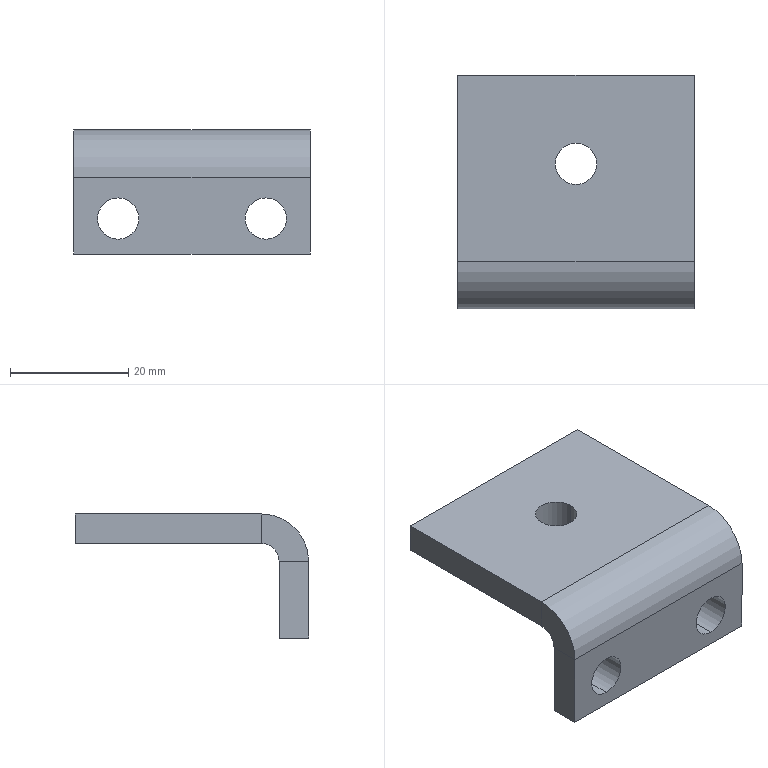Part | SolidWorks | features ICE 2, EdgeFlange 1, Fillet 1, FlatPattern 1, SMBaseFlange 1, SheetMetal 1 | 1 solid | 20 faces | box 40 x 39.5 x 21 mm | volume 10051 mm3 | plane 12 | cylinder 8 | commonest cylinder face diameters 7 x6 6 x1 16 x1
STEP:
#1=CARTESIAN_POINT('',(12.5,-5.,-8.));
#2=VERTEX_POINT('',#1);
#3=CARTESIAN_POINT('',(12.5,-5.,-1.));
#4=VERTEX_POINT('',#3);
#5=CARTESIAN_POINT('',(12.5,-5.,-4.5));
#6=DIRECTION('',(0.,1.,0.));
#7=DIRECTION('',(0.,0.,1.));
#8=AXIS2_PLACEMENT_3D('',#5,#6,#7);
#9=CIRCLE('',#8,3.5);
#10=EDGE_CURVE('',#2,#4,#9,.T.);
#11=ORIENTED_EDGE('',*,*,#10,.F.);
#12=CARTESIAN_POINT('',(12.5,0.,-8.));
#13=VERTEX_POINT('',#12);
#14=CARTESIAN_POINT('',(12.5,-5.,-8.));
#15=DIRECTION('',(0.,1.,0.));
#16=VECTOR('',#15,1000.);
#17=LINE('',#14,#16);
#18=EDGE_CURVE('',#2,#13,#17,.T.);
#19=ORIENTED_EDGE('',*,*,#18,.T.);
#20=CARTESIAN_POINT('',(12.5,0.,-1.));
#21=VERTEX_POINT('',#20);
#22=CARTESIAN_POINT('',(12.5,0.,-4.5));
#23=DIRECTION('',(0.,1.,0.));
#24=DIRECTION('',(0.,0.,1.));
#25=AXIS2_PLACEMENT_3D('',#22,#23,#24);
#26=CIRCLE('',#25,3.5);
#27=EDGE_CURVE('',#13,#21,#26,.T.);
#28=ORIENTED_EDGE('',*,*,#27,.T.);
#29=CARTESIAN_POINT('',(12.5,-5.,-1.));
#30=DIRECTION('',(0.,1.,0.));
#31=VECTOR('',#30,1000.);
#32=LINE('',#29,#31);
#33=EDGE_CURVE('',#4,#21,#32,.T.);
#34=ORIENTED_EDGE('',*,*,#33,.F.);
#35=EDGE_LOOP('',(#11,#19,#28,#34));
#36=FACE_OUTER_BOUND('',#35,.T.);
#37=CARTESIAN_POINT('',(12.5,-5.,-4.5));
#38=DIRECTION('',(0.,1.,0.));
#39=DIRECTION('',(0.,0.,1.));
#40=AXIS2_PLACEMENT_3D('',#37,#38,#39);
#41=CYLINDRICAL_SURFACE('',#40,3.5);
#42=ADVANCED_FACE('',(#36),#41,.F.);
#43=CARTESIAN_POINT('',(-12.5,-5.,-8.));
#44=VERTEX_POINT('',#43);
#45=CARTESIAN_POINT('',(-12.5,-5.,-1.));
#46=VERTEX_POINT('',#45);
#47=CARTESIAN_POINT('',(-12.5,-5.,-4.5));
#48=DIRECTION('',(0.,1.,0.));
#49=DIRECTION('',(0.,0.,1.));
#50=AXIS2_PLACEMENT_3D('',#47,#48,#49);
#51=CIRCLE('',#50,3.5);
#52=EDGE_CURVE('',#44,#46,#51,.T.);
#53=ORIENTED_EDGE('',*,*,#52,.F.);
#54=CARTESIAN_POINT('',(-12.5,0.,-8.));
#55=VERTEX_POINT('',#54);
#56=CARTESIAN_POINT('',(-12.5,-5.,-8.));
#57=DIRECTION('',(0.,1.,0.));
#58=VECTOR('',#57,1000.);
#59=LINE('',#56,#58);
#60=EDGE_CURVE('',#44,#55,#59,.T.);
#61=ORIENTED_EDGE('',*,*,#60,.T.);
#62=CARTESIAN_POINT('',(-12.5,0.,-1.));
#63=VERTEX_POINT('',#62);
#64=CARTESIAN_POINT('',(-12.5,0.,-4.5));
#65=DIRECTION('',(0.,1.,0.));
#66=DIRECTION('',(0.,0.,1.));
#67=AXIS2_PLACEMENT_3D('',#64,#65,#66);
#68=CIRCLE('',#67,3.5);
#69=EDGE_CURVE('',#55,#63,#68,.T.);
#70=ORIENTED_EDGE('',*,*,#69,.T.);
#71=CARTESIAN_POINT('',(-12.5,-5.,-1.));
#72=DIRECTION('',(0.,1.,0.));
#73=VECTOR('',#72,1000.);
#74=LINE('',#71,#73);
#75=EDGE_CURVE('',#46,#63,#74,.T.);
#76=ORIENTED_EDGE('',*,*,#75,.F.);
#77=EDGE_LOOP('',(#53,#61,#70,#76));
#78=FACE_OUTER_BOUND('',#77,.T.);
#79=CARTESIAN_POINT('',(-12.5,-5.,-4.5));
#80=DIRECTION('',(0.,1.,0.));
#81=DIRECTION('',(0.,0.,1.));
#82=AXIS2_PLACEMENT_3D('',#79,#80,#81);
#83=CYLINDRICAL_SURFACE('',#82,3.5);
#84=ADVANCED_FACE('',(#78),#83,.F.);
#85=CARTESIAN_POINT('',(3.5,19.5,10.5));
#86=VERTEX_POINT('',#85);
#87=CARTESIAN_POINT('',(-3.5,19.5,10.5));
#88=VERTEX_POINT('',#87);
#89=CARTESIAN_POINT('',(0.,19.5,10.5));
#90=DIRECTION('',(0.,0.,-1.));
#91=DIRECTION('',(-1.,0.,0.));
#92=AXIS2_PLACEMENT_3D('',#89,#90,#91);
#93=CIRCLE('',#92,3.5);
#94=EDGE_CURVE('',#86,#88,#93,.T.);
#95=ORIENTED_EDGE('',*,*,#94,.F.);
#96=CARTESIAN_POINT('',(3.5,19.5,5.5));
#97=VERTEX_POINT('',#96);
#98=CARTESIAN_POINT('',(3.5,19.5,10.5));
#99=DIRECTION('',(0.,0.,-1.));
#100=VECTOR('',#99,1000.);
#101=LINE('',#98,#100);
#102=EDGE_CURVE('',#86,#97,#101,.T.);
#103=ORIENTED_EDGE('',*,*,#102,.T.);
#104=CARTESIAN_POINT('',(-3.5,19.5,5.5));
#105=VERTEX_POINT('',#104);
#106=CARTESIAN_POINT('',(0.,19.5,5.5));
#107=DIRECTION('',(0.,0.,-1.));
#108=DIRECTION('',(-1.,0.,0.));
#109=AXIS2_PLACEMENT_3D('',#106,#107,#108);
#110=CIRCLE('',#109,3.5);
#111=EDGE_CURVE('',#97,#105,#110,.T.);
#112=ORIENTED_EDGE('',*,*,#111,.T.);
#113=CARTESIAN_POINT('',(-3.5,19.5,10.5));
#114=DIRECTION('',(0.,0.,-1.));
#115=VECTOR('',#114,1000.);
#116=LINE('',#113,#115);
#117=EDGE_CURVE('',#88,#105,#116,.T.);
#118=ORIENTED_EDGE('',*,*,#117,.F.);
#119=EDGE_LOOP('',(#95,#103,#112,#118));
#120=FACE_OUTER_BOUND('',#119,.T.);
#121=CARTESIAN_POINT('',(0.,19.5,10.5));
#122=DIRECTION('',(0.,0.,-1.));
#123=DIRECTION('',(-1.,0.,0.));
#124=AXIS2_PLACEMENT_3D('',#121,#122,#123);
#125=CYLINDRICAL_SURFACE('',#124,3.5);
#126=ADVANCED_FACE('',(#120),#125,.F.);
#127=CARTESIAN_POINT('',(20.,0.,2.5));
#128=VERTEX_POINT('',#127);
#129=CARTESIAN_POINT('',(20.,0.,-10.5));
#130=VERTEX_POINT('',#129);
#131=CARTESIAN_POINT('',(20.,0.,-10.5));
#132=DIRECTION('',(0.,0.,-1.));
#133=VECTOR('',#132,1000.);
#134=LINE('',#131,#133);
#135=EDGE_CURVE('',#128,#130,#134,.T.);
#136=ORIENTED_EDGE('',*,*,#135,.F.);
#137=CARTESIAN_POINT('',(20.,-5.,2.5));
#138=VERTEX_POINT('',#137);
#139=CARTESIAN_POINT('',(20.,0.,2.5));
#140=DIRECTION('',(0.,-1.,0.));
#141=VECTOR('',#140,1000.);
#142=LINE('',#139,#141);
#143=EDGE_CURVE('',#128,#138,#142,.T.);
#144=ORIENTED_EDGE('',*,*,#143,.T.);
#145=CARTESIAN_POINT('',(20.,-5.,-10.5));
#146=VERTEX_POINT('',#145);
#147=CARTESIAN_POINT('',(20.,-5.,-10.5));
#148=DIRECTION('',(0.,0.,-1.));
#149=VECTOR('',#148,1000.);
#150=LINE('',#147,#149);
#151=EDGE_CURVE('',#138,#146,#150,.T.);
#152=ORIENTED_EDGE('',*,*,#151,.T.);
#153=CARTESIAN_POINT('',(20.,-5.,-10.5));
#154=DIRECTION('',(0.,1.,0.));
#155=VECTOR('',#154,1000.);
#156=LINE('',#153,#155);
#157=EDGE_CURVE('',#146,#130,#156,.T.);
#158=ORIENTED_EDGE('',*,*,#157,.T.);
#159=EDGE_LOOP('',(#136,#144,#152,#158));
#160=FACE_OUTER_BOUND('',#159,.T.);
#161=CARTESIAN_POINT('',(20.,-5.,-10.5));
#162=DIRECTION('',(1.,0.,0.));
#163=DIRECTION('',(0.,0.,-1.));
#164=AXIS2_PLACEMENT_3D('',#161,#162,#163);
#165=PLANE('',#164);
#166=ADVANCED_FACE('',(#160),#165,.T.);
#167=CARTESIAN_POINT('',(12.5,-5.,-4.5));
#168=DIRECTION('',(0.,1.,0.));
#169=DIRECTION('',(0.,0.,1.));
#170=AXIS2_PLACEMENT_3D('',#167,#168,#169);
#171=CIRCLE('',#170,3.5);
#172=EDGE_CURVE('',#4,#2,#171,.T.);
#173=ORIENTED_EDGE('',*,*,#172,.T.);
#174=ORIENTED_EDGE('',*,*,#10,.T.);
#175=EDGE_LOOP('',(#173,#174));
#176=FACE_BOUND('',#175,.T.);
#177=CARTESIAN_POINT('',(-12.5,-5.,-4.5));
#178=DIRECTION('',(0.,1.,0.));
#179=DIRECTION('',(0.,0.,1.));
#180=AXIS2_PLACEMENT_3D('',#177,#178,#179);
#181=CIRCLE('',#180,3.5);
#182=EDGE_CURVE('',#46,#44,#181,.T.);
#183=ORIENTED_EDGE('',*,*,#182,.T.);
#184=ORIENTED_EDGE('',*,*,#52,.T.);
#185=EDGE_LOOP('',(#183,#184));
#186=FACE_BOUND('',#185,.T.);
#187=CARTESIAN_POINT('',(-20.,-5.,2.5));
#188=VERTEX_POINT('',#187);
#189=CARTESIAN_POINT('',(20.,-5.,2.5));
#190=DIRECTION('',(-1.,0.,0.));
#191=VECTOR('',#190,1000.);
#192=LINE('',#189,#191);
#193=EDGE_CURVE('',#138,#188,#192,.T.);
#194=ORIENTED_EDGE('',*,*,#193,.T.);
#195=CARTESIAN_POINT('',(-20.,-5.,-10.5));
#196=VERTEX_POINT('',#195);
#197=CARTESIAN_POINT('',(-20.,-5.,-10.5));
#198=DIRECTION('',(0.,0.,1.));
#199=VECTOR('',#198,1000.);
#200=LINE('',#197,#199);
#201=EDGE_CURVE('',#196,#188,#200,.T.);
#202=ORIENTED_EDGE('',*,*,#201,.F.);
#203=CARTESIAN_POINT('',(-20.,-5.,-10.5));
#204=DIRECTION('',(-1.,0.,0.));
#205=VECTOR('',#204,1000.);
#206=LINE('',#203,#205);
#207=EDGE_CURVE('',#146,#196,#206,.T.);
#208=ORIENTED_EDGE('',*,*,#207,.F.);
#209=ORIENTED_EDGE('',*,*,#151,.F.);
#210=EDGE_LOOP('',(#194,#202,#208,#209));
#211=FACE_OUTER_BOUND('',#210,.T.);
#212=CARTESIAN_POINT('',(0.,-5.,0.));
#213=DIRECTION('',(0.,1.,0.));
#214=DIRECTION('',(0.,0.,1.));
#215=AXIS2_PLACEMENT_3D('',#212,#213,#214);
#216=PLANE('',#215);
#217=ADVANCED_FACE('',(#176,#186,#211),#216,.F.);
#218=CARTESIAN_POINT('',(12.5,0.,-4.5));
#219=DIRECTION('',(0.,1.,0.));
#220=DIRECTION('',(0.,0.,1.));
#221=AXIS2_PLACEMENT_3D('',#218,#219,#220);
#222=CIRCLE('',#221,3.5);
#223=EDGE_CURVE('',#21,#13,#222,.T.);
#224=ORIENTED_EDGE('',*,*,#223,.F.);
#225=ORIENTED_EDGE('',*,*,#27,.F.);
#226=EDGE_LOOP('',(#224,#225));
#227=FACE_BOUND('',#226,.T.);
#228=CARTESIAN_POINT('',(-12.5,0.,-4.5));
#229=DIRECTION('',(0.,1.,0.));
#230=DIRECTION('',(0.,0.,1.));
#231=AXIS2_PLACEMENT_3D('',#228,#229,#230);
#232=CIRCLE('',#231,3.5);
#233=EDGE_CURVE('',#63,#55,#232,.T.);
#234=ORIENTED_EDGE('',*,*,#233,.F.);
#235=ORIENTED_EDGE('',*,*,#69,.F.);
#236=EDGE_LOOP('',(#234,#235));
#237=FACE_BOUND('',#236,.T.);
#238=CARTESIAN_POINT('',(-20.,0.,-10.5));
#239=VERTEX_POINT('',#238);
#240=CARTESIAN_POINT('',(-20.,0.,2.5));
#241=VERTEX_POINT('',#240);
#242=CARTESIAN_POINT('',(-20.,0.,-10.5));
#243=DIRECTION('',(0.,0.,1.));
#244=VECTOR('',#243,1000.);
#245=LINE('',#242,#244);
#246=EDGE_CURVE('',#239,#241,#245,.T.);
#247=ORIENTED_EDGE('',*,*,#246,.T.);
#248=CARTESIAN_POINT('',(20.,0.,2.5));
#249=DIRECTION('',(-1.,0.,0.));
#250=VECTOR('',#249,1000.);
#251=LINE('',#248,#250);
#252=EDGE_CURVE('',#128,#241,#251,.T.);
#253=ORIENTED_EDGE('',*,*,#252,.F.);
#254=ORIENTED_EDGE('',*,*,#135,.T.);
#255=CARTESIAN_POINT('',(-20.,0.,-10.5));
#256=DIRECTION('',(-1.,0.,0.));
#257=VECTOR('',#256,1000.);
#258=LINE('',#255,#257);
#259=EDGE_CURVE('',#130,#239,#258,.T.);
#260=ORIENTED_EDGE('',*,*,#259,.T.);
#261=EDGE_LOOP('',(#247,#253,#254,#260));
#262=FACE_OUTER_BOUND('',#261,.T.);
#263=CARTESIAN_POINT('',(0.,0.,0.));
#264=DIRECTION('',(0.,1.,0.));
#265=DIRECTION('',(0.,0.,1.));
#266=AXIS2_PLACEMENT_3D('',#263,#264,#265);
#267=PLANE('',#266);
#268=ADVANCED_FACE('',(#227,#237,#262),#267,.T.);
#269=CARTESIAN_POINT('',(-20.,0.,2.5));
#270=DIRECTION('',(0.,-1.,0.));
#271=VECTOR('',#270,1000.);
#272=LINE('',#269,#271);
#273=EDGE_CURVE('',#241,#188,#272,.T.);
#274=ORIENTED_EDGE('',*,*,#273,.F.);
#275=ORIENTED_EDGE('',*,*,#246,.F.);
#276=CARTESIAN_POINT('',(-20.,-5.,-10.5));
#277=DIRECTION('',(0.,1.,0.));
#278=VECTOR('',#277,1000.);
#279=LINE('',#276,#278);
#280=EDGE_CURVE('',#196,#239,#279,.T.);
#281=ORIENTED_EDGE('',*,*,#280,.F.);
#282=ORIENTED_EDGE('',*,*,#201,.T.);
#283=EDGE_LOOP('',(#274,#275,#281,#282));
#284=FACE_OUTER_BOUND('',#283,.T.);
#285=CARTESIAN_POINT('',(-20.,-5.,-10.5));
#286=DIRECTION('',(-1.,0.,0.));
#287=DIRECTION('',(0.,0.,1.));
#288=AXIS2_PLACEMENT_3D('',#285,#286,#287);
#289=PLANE('',#288);
#290=ADVANCED_FACE('',(#284),#289,.T.);
#291=ORIENTED_EDGE('',*,*,#259,.F.);
#292=ORIENTED_EDGE('',*,*,#157,.F.);
#293=ORIENTED_EDGE('',*,*,#207,.T.);
#294=ORIENTED_EDGE('',*,*,#280,.T.);
#295=EDGE_LOOP('',(#291,#292,#293,#294));
#296=FACE_OUTER_BOUND('',#295,.T.);
#297=CARTESIAN_POINT('',(-20.,-5.,-10.5));
#298=DIRECTION('',(0.,0.,-1.));
#299=DIRECTION('',(-1.,0.,0.));
#300=AXIS2_PLACEMENT_3D('',#297,#298,#299);
#301=PLANE('',#300);
#302=ADVANCED_FACE('',(#296),#301,.T.);
#303=CARTESIAN_POINT('',(-20.,3.,5.5));
#304=VERTEX_POINT('',#303);
#305=CARTESIAN_POINT('',(-20.,3.,10.5));
#306=VERTEX_POINT('',#305);
#307=CARTESIAN_POINT('',(-20.,3.,10.5));
#308=DIRECTION('',(0.,0.,1.));
#309=VECTOR('',#308,1000.);
#310=LINE('',#307,#309);
#311=EDGE_CURVE('',#304,#306,#310,.T.);
#312=ORIENTED_EDGE('',*,*,#311,.F.);
#313=CARTESIAN_POINT('',(-20.,3.,2.5));
#314=DIRECTION('',(-1.,0.,0.));
#315=DIRECTION('',(0.,0.,-1.));
#316=AXIS2_PLACEMENT_3D('',#313,#314,#315);
#317=CIRCLE('',#316,3.);
#318=EDGE_CURVE('',#241,#304,#317,.T.);
#319=ORIENTED_EDGE('',*,*,#318,.F.);
#320=ORIENTED_EDGE('',*,*,#273,.T.);
#321=CARTESIAN_POINT('',(-20.,3.,2.5));
#322=DIRECTION('',(-1.,0.,0.));
#323=DIRECTION('',(0.,0.,-1.));
#324=AXIS2_PLACEMENT_3D('',#321,#322,#323);
#325=CIRCLE('',#324,8.);
#326=EDGE_CURVE('',#188,#306,#325,.T.);
#327=ORIENTED_EDGE('',*,*,#326,.T.);
#328=EDGE_LOOP('',(#312,#319,#320,#327));
#329=FACE_OUTER_BOUND('',#328,.T.);
#330=CARTESIAN_POINT('',(-20.,3.,2.5));
#331=DIRECTION('',(-1.,0.,0.));
#332=DIRECTION('',(0.,0.,1.));
#333=AXIS2_PLACEMENT_3D('',#330,#331,#332);
#334=PLANE('',#333);
#335=ADVANCED_FACE('',(#329),#334,.T.);
#336=CARTESIAN_POINT('',(20.,3.,5.5));
#337=VERTEX_POINT('',#336);
#338=CARTESIAN_POINT('',(20.,3.,2.5));
#339=DIRECTION('',(1.,0.,0.));
#340=DIRECTION('',(0.,0.,-1.));
#341=AXIS2_PLACEMENT_3D('',#338,#339,#340);
#342=CIRCLE('',#341,3.);
#343=EDGE_CURVE('',#337,#128,#342,.T.);
#344=ORIENTED_EDGE('',*,*,#343,.F.);
#345=CARTESIAN_POINT('',(20.,3.,10.5));
#346=VERTEX_POINT('',#345);
#347=CARTESIAN_POINT('',(20.,3.,5.5));
#348=DIRECTION('',(0.,0.,1.));
#349=VECTOR('',#348,1000.);
#350=LINE('',#347,#349);
#351=EDGE_CURVE('',#337,#346,#350,.T.);
#352=ORIENTED_EDGE('',*,*,#351,.T.);
#353=CARTESIAN_POINT('',(20.,3.,2.5));
#354=DIRECTION('',(1.,0.,0.));
#355=DIRECTION('',(0.,0.,-1.));
#356=AXIS2_PLACEMENT_3D('',#353,#354,#355);
#357=CIRCLE('',#356,8.);
#358=EDGE_CURVE('',#346,#138,#357,.T.);
#359=ORIENTED_EDGE('',*,*,#358,.T.);
#360=ORIENTED_EDGE('',*,*,#143,.F.);
#361=EDGE_LOOP('',(#344,#352,#359,#360));
#362=FACE_OUTER_BOUND('',#361,.T.);
#363=CARTESIAN_POINT('',(20.,3.,2.5));
#364=DIRECTION('',(-1.,0.,0.));
#365=DIRECTION('',(0.,0.,1.));
#366=AXIS2_PLACEMENT_3D('',#363,#364,#365);
#367=PLANE('',#366);
#368=ADVANCED_FACE('',(#362),#367,.F.);
#369=ORIENTED_EDGE('',*,*,#193,.F.);
#370=ORIENTED_EDGE('',*,*,#358,.F.);
#371=CARTESIAN_POINT('',(-20.,3.,10.5));
#372=DIRECTION('',(-1.,0.,0.));
#373=VECTOR('',#372,1000.);
#374=LINE('',#371,#373);
#375=EDGE_CURVE('',#346,#306,#374,.T.);
#376=ORIENTED_EDGE('',*,*,#375,.T.);
#377=ORIENTED_EDGE('',*,*,#326,.F.);
#378=EDGE_LOOP('',(#369,#370,#376,#377));
#379=FACE_OUTER_BOUND('',#378,.T.);
#380=CARTESIAN_POINT('',(20.,3.,2.5));
#381=DIRECTION('',(1.,0.,0.));
#382=DIRECTION('',(0.,0.,1.));
#383=AXIS2_PLACEMENT_3D('',#380,#381,#382);
#384=CYLINDRICAL_SURFACE('',#383,8.);
#385=ADVANCED_FACE('',(#379),#384,.T.);
#386=ORIENTED_EDGE('',*,*,#252,.T.);
#387=ORIENTED_EDGE('',*,*,#318,.T.);
#388=CARTESIAN_POINT('',(-20.,3.,5.5));
#389=DIRECTION('',(1.,0.,0.));
#390=VECTOR('',#389,1000.);
#391=LINE('',#388,#390);
#392=EDGE_CURVE('',#304,#337,#391,.T.);
#393=ORIENTED_EDGE('',*,*,#392,.T.);
#394=ORIENTED_EDGE('',*,*,#343,.T.);
#395=EDGE_LOOP('',(#386,#387,#393,#394));
#396=FACE_OUTER_BOUND('',#395,.T.);
#397=CARTESIAN_POINT('',(20.,3.,2.5));
#398=DIRECTION('',(1.,0.,0.));
#399=DIRECTION('',(0.,0.,1.));
#400=AXIS2_PLACEMENT_3D('',#397,#398,#399);
#401=CYLINDRICAL_SURFACE('',#400,3.);
#402=ADVANCED_FACE('',(#396),#401,.F.);
#403=ORIENTED_EDGE('',*,*,#311,.T.);
#404=CARTESIAN_POINT('',(-20.,34.5,10.5));
#405=VERTEX_POINT('',#404);
#406=CARTESIAN_POINT('',(-20.,0.,10.5));
#407=DIRECTION('',(0.,-1.,0.));
#408=VECTOR('',#407,1000.);
#409=LINE('',#406,#408);
#410=EDGE_CURVE('',#405,#306,#409,.T.);
#411=ORIENTED_EDGE('',*,*,#410,.F.);
#412=CARTESIAN_POINT('',(-20.,34.5,5.5));
#413=VERTEX_POINT('',#412);
#414=CARTESIAN_POINT('',(-20.,34.5,10.5));
#415=DIRECTION('',(0.,0.,-1.));
#416=VECTOR('',#415,1000.);
#417=LINE('',#414,#416);
#418=EDGE_CURVE('',#405,#413,#417,.T.);
#419=ORIENTED_EDGE('',*,*,#418,.T.);
#420=CARTESIAN_POINT('',(-20.,0.,5.5));
#421=DIRECTION('',(0.,-1.,0.));
#422=VECTOR('',#421,1000.);
#423=LINE('',#420,#422);
#424=EDGE_CURVE('',#413,#304,#423,.T.);
#425=ORIENTED_EDGE('',*,*,#424,.T.);
#426=EDGE_LOOP('',(#403,#411,#419,#425));
#427=FACE_OUTER_BOUND('',#426,.T.);
#428=CARTESIAN_POINT('',(-20.,0.,10.5));
#429=DIRECTION('',(1.,0.,0.));
#430=DIRECTION('',(0.,0.,-1.));
#431=AXIS2_PLACEMENT_3D('',#428,#429,#430);
#432=PLANE('',#431);
#433=ADVANCED_FACE('',(#427),#432,.F.);
#434=ORIENTED_EDGE('',*,*,#351,.F.);
#435=CARTESIAN_POINT('',(20.,34.5,5.5));
#436=VERTEX_POINT('',#435);
#437=CARTESIAN_POINT('',(20.,34.5,5.5));
#438=DIRECTION('',(0.,1.,0.));
#439=VECTOR('',#438,1000.);
#440=LINE('',#437,#439);
#441=EDGE_CURVE('',#337,#436,#440,.T.);
#442=ORIENTED_EDGE('',*,*,#441,.T.);
#443=CARTESIAN_POINT('',(20.,34.5,10.5));
#444=VERTEX_POINT('',#443);
#445=CARTESIAN_POINT('',(20.,34.5,10.5));
#446=DIRECTION('',(0.,0.,-1.));
#447=VECTOR('',#446,1000.);
#448=LINE('',#445,#447);
#449=EDGE_CURVE('',#444,#436,#448,.T.);
#450=ORIENTED_EDGE('',*,*,#449,.F.);
#451=CARTESIAN_POINT('',(20.,0.,10.5));
#452=DIRECTION('',(0.,1.,0.));
#453=VECTOR('',#452,1000.);
#454=LINE('',#451,#453);
#455=EDGE_CURVE('',#346,#444,#454,.T.);
#456=ORIENTED_EDGE('',*,*,#455,.F.);
#457=EDGE_LOOP('',(#434,#442,#450,#456));
#458=FACE_OUTER_BOUND('',#457,.T.);
#459=CARTESIAN_POINT('',(20.,34.5,10.5));
#460=DIRECTION('',(-1.,0.,0.));
#461=DIRECTION('',(0.,0.,1.));
#462=AXIS2_PLACEMENT_3D('',#459,#460,#461);
#463=PLANE('',#462);
#464=ADVANCED_FACE('',(#458),#463,.F.);
#465=CARTESIAN_POINT('',(0.,19.5,10.5));
#466=DIRECTION('',(0.,0.,-1.));
#467=DIRECTION('',(-1.,0.,0.));
#468=AXIS2_PLACEMENT_3D('',#465,#466,#467);
#469=CIRCLE('',#468,3.5);
#470=EDGE_CURVE('',#88,#86,#469,.T.);
#471=ORIENTED_EDGE('',*,*,#470,.T.);
#472=ORIENTED_EDGE('',*,*,#94,.T.);
#473=EDGE_LOOP('',(#471,#472));
#474=FACE_BOUND('',#473,.T.);
#475=ORIENTED_EDGE('',*,*,#375,.F.);
#476=ORIENTED_EDGE('',*,*,#455,.T.);
#477=CARTESIAN_POINT('',(0.,34.5,10.5));
#478=DIRECTION('',(-1.,0.,0.));
#479=VECTOR('',#478,1000.);
#480=LINE('',#477,#479);
#481=EDGE_CURVE('',#444,#405,#480,.T.);
#482=ORIENTED_EDGE('',*,*,#481,.T.);
#483=ORIENTED_EDGE('',*,*,#410,.T.);
#484=EDGE_LOOP('',(#475,#476,#482,#483));
#485=FACE_OUTER_BOUND('',#484,.T.);
#486=CARTESIAN_POINT('',(0.,0.,10.5));
#487=DIRECTION('',(0.,0.,-1.));
#488=DIRECTION('',(-1.,0.,0.));
#489=AXIS2_PLACEMENT_3D('',#486,#487,#488);
#490=PLANE('',#489);
#491=ADVANCED_FACE('',(#474,#485),#490,.F.);
#492=CARTESIAN_POINT('',(0.,19.5,5.5));
#493=DIRECTION('',(0.,0.,-1.));
#494=DIRECTION('',(-1.,0.,0.));
#495=AXIS2_PLACEMENT_3D('',#492,#493,#494);
#496=CIRCLE('',#495,3.5);
#497=EDGE_CURVE('',#105,#97,#496,.T.);
#498=ORIENTED_EDGE('',*,*,#497,.F.);
#499=ORIENTED_EDGE('',*,*,#111,.F.);
#500=EDGE_LOOP('',(#498,#499));
#501=FACE_BOUND('',#500,.T.);
#502=ORIENTED_EDGE('',*,*,#441,.F.);
#503=ORIENTED_EDGE('',*,*,#392,.F.);
#504=ORIENTED_EDGE('',*,*,#424,.F.);
#505=CARTESIAN_POINT('',(-20.,34.5,5.5));
#506=DIRECTION('',(-1.,0.,0.));
#507=VECTOR('',#506,1000.);
#508=LINE('',#505,#507);
#509=EDGE_CURVE('',#436,#413,#508,.T.);
#510=ORIENTED_EDGE('',*,*,#509,.F.);
#511=EDGE_LOOP('',(#502,#503,#504,#510));
#512=FACE_OUTER_BOUND('',#511,.T.);
#513=CARTESIAN_POINT('',(0.,0.,5.5));
#514=DIRECTION('',(0.,0.,-1.));
#515=DIRECTION('',(-1.,0.,0.));
#516=AXIS2_PLACEMENT_3D('',#513,#514,#515);
#517=PLANE('',#516);
#518=ADVANCED_FACE('',(#501,#512),#517,.T.);
#519=ORIENTED_EDGE('',*,*,#509,.T.);
#520=ORIENTED_EDGE('',*,*,#418,.F.);
#521=ORIENTED_EDGE('',*,*,#481,.F.);
#522=ORIENTED_EDGE('',*,*,#449,.T.);
#523=EDGE_LOOP('',(#519,#520,#521,#522));
#524=FACE_OUTER_BOUND('',#523,.T.);
#525=CARTESIAN_POINT('',(-20.,34.5,10.5));
#526=DIRECTION('',(0.,-1.,0.));
#527=DIRECTION('',(0.,0.,-1.));
#528=AXIS2_PLACEMENT_3D('',#525,#526,#527);
#529=PLANE('',#528);
#530=ADVANCED_FACE('',(#524),#529,.F.);
#531=ORIENTED_EDGE('',*,*,#102,.F.);
#532=ORIENTED_EDGE('',*,*,#470,.F.);
#533=ORIENTED_EDGE('',*,*,#117,.T.);
#534=ORIENTED_EDGE('',*,*,#497,.T.);
#535=EDGE_LOOP('',(#531,#532,#533,#534));
#536=FACE_OUTER_BOUND('',#535,.T.);
#537=CARTESIAN_POINT('',(0.,19.5,10.5));
#538=DIRECTION('',(0.,0.,-1.));
#539=DIRECTION('',(-1.,0.,0.));
#540=AXIS2_PLACEMENT_3D('',#537,#538,#539);
#541=CYLINDRICAL_SURFACE('',#540,3.5);
#542=ADVANCED_FACE('',(#536),#541,.F.);
#543=ORIENTED_EDGE('',*,*,#60,.F.);
#544=ORIENTED_EDGE('',*,*,#182,.F.);
#545=ORIENTED_EDGE('',*,*,#75,.T.);
#546=ORIENTED_EDGE('',*,*,#233,.T.);
#547=EDGE_LOOP('',(#543,#544,#545,#546));
#548=FACE_OUTER_BOUND('',#547,.T.);
#549=CARTESIAN_POINT('',(-12.5,-5.,-4.5));
#550=DIRECTION('',(0.,1.,0.));
#551=DIRECTION('',(0.,0.,1.));
#552=AXIS2_PLACEMENT_3D('',#549,#550,#551);
#553=CYLINDRICAL_SURFACE('',#552,3.5);
#554=ADVANCED_FACE('',(#548),#553,.F.);
#555=ORIENTED_EDGE('',*,*,#18,.F.);
#556=ORIENTED_EDGE('',*,*,#172,.F.);
#557=ORIENTED_EDGE('',*,*,#33,.T.);
#558=ORIENTED_EDGE('',*,*,#223,.T.);
#559=EDGE_LOOP('',(#555,#556,#557,#558));
#560=FACE_OUTER_BOUND('',#559,.T.);
#561=CARTESIAN_POINT('',(12.5,-5.,-4.5));
#562=DIRECTION('',(0.,1.,0.));
#563=DIRECTION('',(0.,0.,1.));
#564=AXIS2_PLACEMENT_3D('',#561,#562,#563);
#565=CYLINDRICAL_SURFACE('',#564,3.5);
#566=ADVANCED_FACE('',(#560),#565,.F.);
#567=CLOSED_SHELL('',(#42,#84,#126,#166,#217,#268,#290,#302,#335,#368,#385,#402,#433,#464,#491,#518,#530,#542,#554,#566));
#568=MANIFOLD_SOLID_BREP('',#567);
#569=CARTESIAN_POINT('',(0.,0.,0.));
#570=DIRECTION('',(0.,0.,1.));
#571=DIRECTION('',(1.,0.,0.));
#572=AXIS2_PLACEMENT_3D('',#569,#570,#571);
#573=(LENGTH_UNIT()NAMED_UNIT(*)SI_UNIT(.MILLI.,.METRE.));
#574=UNCERTAINTY_MEASURE_WITH_UNIT(LENGTH_MEASURE(0.00001),#573,'','');
#575=(NAMED_UNIT(*)PLANE_ANGLE_UNIT()SI_UNIT($,.RADIAN.));
#576=(NAMED_UNIT(*)SI_UNIT($,.STERADIAN.)SOLID_ANGLE_UNIT());
#577=(GEOMETRIC_REPRESENTATION_CONTEXT(3)GLOBAL_UNCERTAINTY_ASSIGNED_CONTEXT((#574))GLOBAL_UNIT_ASSIGNED_CONTEXT((#573,#575,#576))REPRESENTATION_CONTEXT('',''));
#578=ADVANCED_BREP_SHAPE_REPRESENTATION('',(#568,#572),#577);